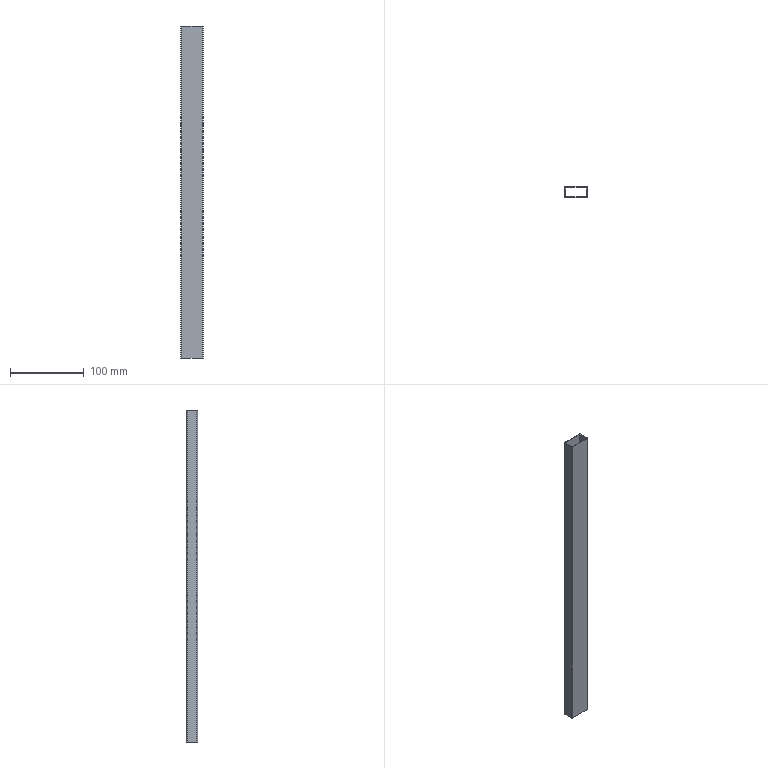Part | STEP file | Q7C1210 | 1 solid | 18 faces | box 30 x 15 x 450 mm | volume 38263 mm3 | plane 10 | cylinder 8 | commonest cylinder face diameters 2 x4 4 x4